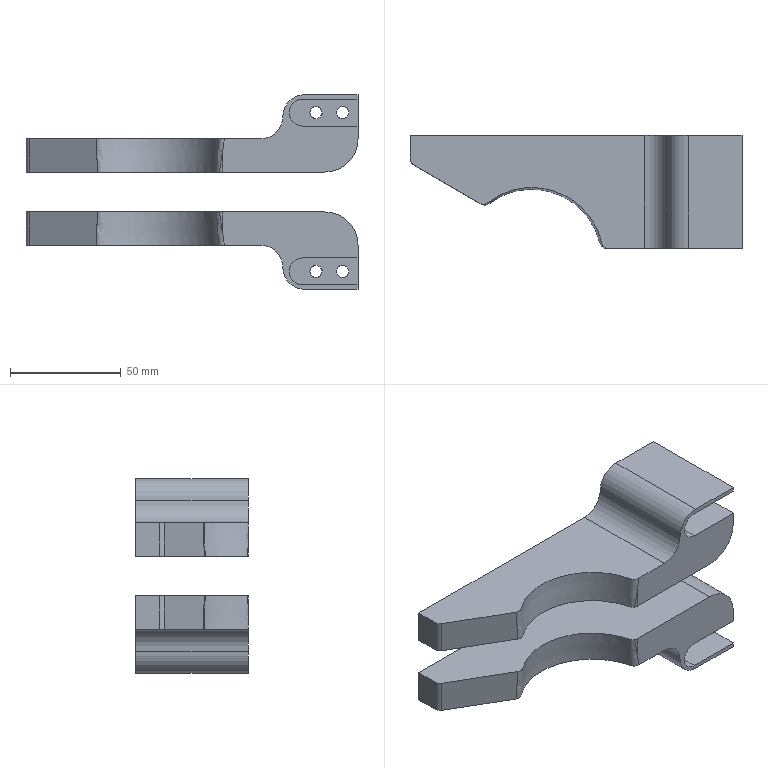NC program | NX | posted with a generic post | part box 150 x 51 x 88 mm
Lines 1 to 42 of 21241:
N10 G17 G21 G94 G90
(FLOOR_WALL , TOOL : D63)
N12 T01 M6
N14 G54
N16 G17 G0 G90 X112.499 Y0. S6500 M3
N18 G43 Z30. H1
N20 Z3.
N22 G94 G1 Z0. F1500.
N24 X109.499
N26 X-109.5
N28 X-112.5
N30 Z3.
N32 G0 Z30.
N34 M5
(DRILLING , TOOL : D6A45)
N36 T07 M6
N38 G54
N40 G17 G0 G90 X56. Y9.4 S5000 M3
N42 G43 Z30. H7
N44 G94 G81 G98 Z-1. F250. R3.
N46 X68.
N48 G80
N50 G0 X68. Y9.4 Z30.
N52 M5
(DRILLING_COPY , TOOL : 5.5ZT)
N54 T15 M6
N56 G54
N58 G17 G0 G90 X56. Y9.4 S2000 M3
N60 G43 Z30. H15
N62 G94 G83 G98 Z-53.652 F120. Q2. R3.
N64 X68.
N66 G80
N68 G0 X68. Y9.4 Z30.
N70 M5